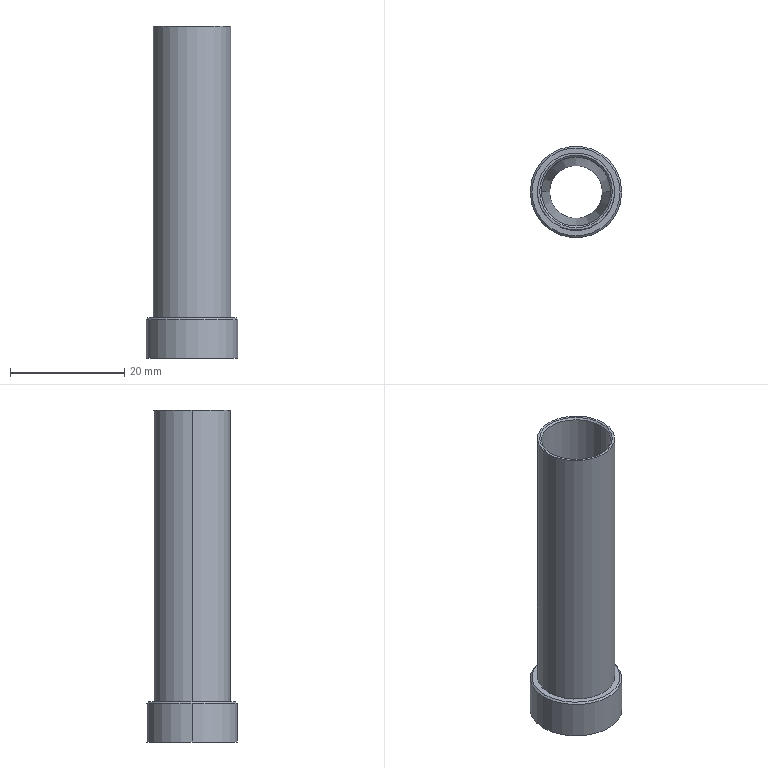Part | SolidWorks | features Chamfer 3, ICE 3, Extrusion 1 | 1 solid | 20 faces | box 16 x 16 x 58 mm | volume 2465 mm3 | cylinder 10 | cone 6 | plane 4 | commonest cylinder face diameters 9.2 x2 12.1 x2 12.5 x2 13.5 x2 16 x2
STEP:
#1=CARTESIAN_POINT('',(-6.05,0.,57.7));
#2=VERTEX_POINT('',#1);
#3=CARTESIAN_POINT('',(6.05,0.,57.7));
#4=VERTEX_POINT('',#3);
#5=CARTESIAN_POINT('',(0.,0.,57.7));
#6=DIRECTION('',(0.,0.,1.));
#7=DIRECTION('',(1.,0.,0.));
#8=AXIS2_PLACEMENT_3D('',#5,#6,#7);
#9=CIRCLE('',#8,6.05);
#10=EDGE_CURVE('',#2,#4,#9,.T.);
#11=ORIENTED_EDGE('',*,*,#10,.F.);
#12=CARTESIAN_POINT('',(-6.35,0.,58.));
#13=VERTEX_POINT('',#12);
#14=CARTESIAN_POINT('',(-6.05,0.,57.7));
#15=DIRECTION('',(-0.7071,0.,0.7071));
#16=VECTOR('',#15,1000.);
#17=LINE('',#14,#16);
#18=EDGE_CURVE('',#2,#13,#17,.T.);
#19=ORIENTED_EDGE('',*,*,#18,.T.);
#20=CARTESIAN_POINT('',(6.35,0.,58.));
#21=VERTEX_POINT('',#20);
#22=CARTESIAN_POINT('',(0.,0.,58.));
#23=DIRECTION('',(0.,0.,-1.));
#24=DIRECTION('',(1.,0.,0.));
#25=AXIS2_PLACEMENT_3D('',#22,#23,#24);
#26=CIRCLE('',#25,6.35);
#27=EDGE_CURVE('',#21,#13,#26,.T.);
#28=ORIENTED_EDGE('',*,*,#27,.F.);
#29=CARTESIAN_POINT('',(6.05,0.,57.7));
#30=DIRECTION('',(0.7071,0.,0.7071));
#31=VECTOR('',#30,1000.);
#32=LINE('',#29,#31);
#33=EDGE_CURVE('',#4,#21,#32,.T.);
#34=ORIENTED_EDGE('',*,*,#33,.F.);
#35=EDGE_LOOP('',(#11,#19,#28,#34));
#36=FACE_OUTER_BOUND('',#35,.T.);
#37=CARTESIAN_POINT('',(0.,0.,57.7));
#38=DIRECTION('',(0.,0.,1.));
#39=DIRECTION('',(1.,0.,0.));
#40=AXIS2_PLACEMENT_3D('',#37,#38,#39);
#41=CONICAL_SURFACE('',#40,6.05,0.7854);
#42=ADVANCED_FACE('',(#36),#41,.F.);
#43=CARTESIAN_POINT('',(-4.6,0.,8.));
#44=VERTEX_POINT('',#43);
#45=CARTESIAN_POINT('',(4.6,0.,8.));
#46=VERTEX_POINT('',#45);
#47=CARTESIAN_POINT('',(0.,0.,8.));
#48=DIRECTION('',(0.,0.,1.));
#49=DIRECTION('',(1.,0.,0.));
#50=AXIS2_PLACEMENT_3D('',#47,#48,#49);
#51=CIRCLE('',#50,4.6);
#52=EDGE_CURVE('',#44,#46,#51,.T.);
#53=ORIENTED_EDGE('',*,*,#52,.F.);
#54=CARTESIAN_POINT('',(-6.05,0.,23.));
#55=VERTEX_POINT('',#54);
#56=CARTESIAN_POINT('',(-4.6,0.,8.));
#57=DIRECTION('',(-0.09622,0.,0.9954));
#58=VECTOR('',#57,1000.);
#59=LINE('',#56,#58);
#60=EDGE_CURVE('',#44,#55,#59,.T.);
#61=ORIENTED_EDGE('',*,*,#60,.T.);
#62=CARTESIAN_POINT('',(6.05,0.,23.));
#63=VERTEX_POINT('',#62);
#64=CARTESIAN_POINT('',(0.,0.,23.));
#65=DIRECTION('',(0.,0.,1.));
#66=DIRECTION('',(1.,0.,0.));
#67=AXIS2_PLACEMENT_3D('',#64,#65,#66);
#68=CIRCLE('',#67,6.05);
#69=EDGE_CURVE('',#55,#63,#68,.T.);
#70=ORIENTED_EDGE('',*,*,#69,.T.);
#71=CARTESIAN_POINT('',(4.6,0.,8.));
#72=DIRECTION('',(0.09622,0.,0.9954));
#73=VECTOR('',#72,1000.);
#74=LINE('',#71,#73);
#75=EDGE_CURVE('',#46,#63,#74,.T.);
#76=ORIENTED_EDGE('',*,*,#75,.F.);
#77=EDGE_LOOP('',(#53,#61,#70,#76));
#78=FACE_OUTER_BOUND('',#77,.T.);
#79=CARTESIAN_POINT('',(0.,0.,8.));
#80=DIRECTION('',(0.,0.,1.));
#81=DIRECTION('',(1.,0.,0.));
#82=AXIS2_PLACEMENT_3D('',#79,#80,#81);
#83=CONICAL_SURFACE('',#82,4.6,0.09637);
#84=ADVANCED_FACE('',(#78),#83,.F.);
#85=ORIENTED_EDGE('',*,*,#69,.F.);
#86=CARTESIAN_POINT('',(-6.05,0.,23.));
#87=DIRECTION('',(0.,0.,1.));
#88=VECTOR('',#87,1000.);
#89=LINE('',#86,#88);
#90=EDGE_CURVE('',#55,#2,#89,.T.);
#91=ORIENTED_EDGE('',*,*,#90,.T.);
#92=ORIENTED_EDGE('',*,*,#10,.T.);
#93=CARTESIAN_POINT('',(6.05,0.,23.));
#94=DIRECTION('',(0.,0.,1.));
#95=VECTOR('',#94,1000.);
#96=LINE('',#93,#95);
#97=EDGE_CURVE('',#63,#4,#96,.T.);
#98=ORIENTED_EDGE('',*,*,#97,.F.);
#99=EDGE_LOOP('',(#85,#91,#92,#98));
#100=FACE_OUTER_BOUND('',#99,.T.);
#101=CARTESIAN_POINT('',(0.,0.,23.));
#102=DIRECTION('',(0.,0.,1.));
#103=DIRECTION('',(1.,0.,0.));
#104=AXIS2_PLACEMENT_3D('',#101,#102,#103);
#105=CYLINDRICAL_SURFACE('',#104,6.05);
#106=ADVANCED_FACE('',(#100),#105,.F.);
#107=CARTESIAN_POINT('',(7.7,0.,7.));
#108=VERTEX_POINT('',#107);
#109=CARTESIAN_POINT('',(-7.7,0.,7.));
#110=VERTEX_POINT('',#109);
#111=CARTESIAN_POINT('',(0.,0.,7.));
#112=DIRECTION('',(0.,0.,1.));
#113=DIRECTION('',(-1.,0.,0.));
#114=AXIS2_PLACEMENT_3D('',#111,#112,#113);
#115=CIRCLE('',#114,7.7);
#116=EDGE_CURVE('',#108,#110,#115,.T.);
#117=ORIENTED_EDGE('',*,*,#116,.F.);
#118=CARTESIAN_POINT('',(8.,0.,6.7));
#119=VERTEX_POINT('',#118);
#120=CARTESIAN_POINT('',(8.,0.,6.7));
#121=DIRECTION('',(0.7071,0.,-0.7071));
#122=VECTOR('',#121,1000.);
#123=LINE('',#120,#122);
#124=EDGE_CURVE('',#108,#119,#123,.T.);
#125=ORIENTED_EDGE('',*,*,#124,.T.);
#126=CARTESIAN_POINT('',(-8.,0.,6.7));
#127=VERTEX_POINT('',#126);
#128=CARTESIAN_POINT('',(0.,0.,6.7));
#129=DIRECTION('',(0.,0.,-1.));
#130=DIRECTION('',(-1.,0.,0.));
#131=AXIS2_PLACEMENT_3D('',#128,#129,#130);
#132=CIRCLE('',#131,8.);
#133=EDGE_CURVE('',#127,#119,#132,.T.);
#134=ORIENTED_EDGE('',*,*,#133,.F.);
#135=CARTESIAN_POINT('',(-8.,0.,6.7));
#136=DIRECTION('',(-0.7071,0.,-0.7071));
#137=VECTOR('',#136,1000.);
#138=LINE('',#135,#137);
#139=EDGE_CURVE('',#110,#127,#138,.T.);
#140=ORIENTED_EDGE('',*,*,#139,.F.);
#141=EDGE_LOOP('',(#117,#125,#134,#140));
#142=FACE_OUTER_BOUND('',#141,.T.);
#143=CARTESIAN_POINT('',(0.,0.,6.7));
#144=DIRECTION('',(0.,0.,-1.));
#145=DIRECTION('',(-1.,0.,0.));
#146=AXIS2_PLACEMENT_3D('',#143,#144,#145);
#147=CONICAL_SURFACE('',#146,8.,0.7854);
#148=ADVANCED_FACE('',(#142),#147,.T.);
#149=ORIENTED_EDGE('',*,*,#133,.T.);
#150=CARTESIAN_POINT('',(8.,0.,0.));
#151=VERTEX_POINT('',#150);
#152=CARTESIAN_POINT('',(8.,0.,7.));
#153=DIRECTION('',(0.,0.,-1.));
#154=VECTOR('',#153,1000.);
#155=LINE('',#152,#154);
#156=EDGE_CURVE('',#119,#151,#155,.T.);
#157=ORIENTED_EDGE('',*,*,#156,.T.);
#158=CARTESIAN_POINT('',(-8.,0.,0.));
#159=VERTEX_POINT('',#158);
#160=CARTESIAN_POINT('',(0.,0.,0.));
#161=DIRECTION('',(0.,0.,-1.));
#162=DIRECTION('',(-1.,0.,0.));
#163=AXIS2_PLACEMENT_3D('',#160,#161,#162);
#164=CIRCLE('',#163,8.);
#165=EDGE_CURVE('',#159,#151,#164,.T.);
#166=ORIENTED_EDGE('',*,*,#165,.F.);
#167=CARTESIAN_POINT('',(-8.,0.,7.));
#168=DIRECTION('',(0.,0.,-1.));
#169=VECTOR('',#168,1000.);
#170=LINE('',#167,#169);
#171=EDGE_CURVE('',#127,#159,#170,.T.);
#172=ORIENTED_EDGE('',*,*,#171,.F.);
#173=EDGE_LOOP('',(#149,#157,#166,#172));
#174=FACE_OUTER_BOUND('',#173,.T.);
#175=CARTESIAN_POINT('',(0.,0.,7.));
#176=DIRECTION('',(0.,0.,-1.));
#177=DIRECTION('',(-1.,0.,0.));
#178=AXIS2_PLACEMENT_3D('',#175,#176,#177);
#179=CYLINDRICAL_SURFACE('',#178,8.);
#180=ADVANCED_FACE('',(#174),#179,.T.);
#181=CARTESIAN_POINT('',(6.25,0.,6.));
#182=VERTEX_POINT('',#181);
#183=CARTESIAN_POINT('',(-6.25,0.,6.));
#184=VERTEX_POINT('',#183);
#185=CARTESIAN_POINT('',(0.,0.,6.));
#186=DIRECTION('',(0.,0.,-1.));
#187=DIRECTION('',(-1.,0.,0.));
#188=AXIS2_PLACEMENT_3D('',#185,#186,#187);
#189=CIRCLE('',#188,6.25);
#190=EDGE_CURVE('',#182,#184,#189,.T.);
#191=ORIENTED_EDGE('',*,*,#190,.F.);
#192=CARTESIAN_POINT('',(6.25,0.,0.));
#193=VERTEX_POINT('',#192);
#194=CARTESIAN_POINT('',(6.25,0.,6.));
#195=DIRECTION('',(0.,0.,-1.));
#196=VECTOR('',#195,1000.);
#197=LINE('',#194,#196);
#198=EDGE_CURVE('',#182,#193,#197,.T.);
#199=ORIENTED_EDGE('',*,*,#198,.T.);
#200=CARTESIAN_POINT('',(-6.25,0.,0.));
#201=VERTEX_POINT('',#200);
#202=CARTESIAN_POINT('',(0.,0.,0.));
#203=DIRECTION('',(0.,0.,-1.));
#204=DIRECTION('',(-1.,0.,0.));
#205=AXIS2_PLACEMENT_3D('',#202,#203,#204);
#206=CIRCLE('',#205,6.25);
#207=EDGE_CURVE('',#193,#201,#206,.T.);
#208=ORIENTED_EDGE('',*,*,#207,.T.);
#209=CARTESIAN_POINT('',(-6.25,0.,6.));
#210=DIRECTION('',(0.,0.,-1.));
#211=VECTOR('',#210,1000.);
#212=LINE('',#209,#211);
#213=EDGE_CURVE('',#184,#201,#212,.T.);
#214=ORIENTED_EDGE('',*,*,#213,.F.);
#215=EDGE_LOOP('',(#191,#199,#208,#214));
#216=FACE_OUTER_BOUND('',#215,.T.);
#217=CARTESIAN_POINT('',(0.,0.,6.));
#218=DIRECTION('',(0.,0.,-1.));
#219=DIRECTION('',(-1.,0.,0.));
#220=AXIS2_PLACEMENT_3D('',#217,#218,#219);
#221=CYLINDRICAL_SURFACE('',#220,6.25);
#222=ADVANCED_FACE('',(#216),#221,.F.);
#223=CARTESIAN_POINT('',(6.75,0.,58.));
#224=VERTEX_POINT('',#223);
#225=CARTESIAN_POINT('',(-6.75,0.,58.));
#226=VERTEX_POINT('',#225);
#227=CARTESIAN_POINT('',(0.,0.,58.));
#228=DIRECTION('',(0.,0.,1.));
#229=DIRECTION('',(1.,0.,0.));
#230=AXIS2_PLACEMENT_3D('',#227,#228,#229);
#231=CIRCLE('',#230,6.75);
#232=EDGE_CURVE('',#224,#226,#231,.T.);
#233=ORIENTED_EDGE('',*,*,#232,.F.);
#234=CARTESIAN_POINT('',(6.75,0.,7.));
#235=VERTEX_POINT('',#234);
#236=CARTESIAN_POINT('',(6.75,0.,58.));
#237=DIRECTION('',(0.,0.,-1.));
#238=VECTOR('',#237,1000.);
#239=LINE('',#236,#238);
#240=EDGE_CURVE('',#224,#235,#239,.T.);
#241=ORIENTED_EDGE('',*,*,#240,.T.);
#242=CARTESIAN_POINT('',(-6.75,0.,7.));
#243=VERTEX_POINT('',#242);
#244=CARTESIAN_POINT('',(0.,0.,7.));
#245=DIRECTION('',(0.,0.,-1.));
#246=DIRECTION('',(-1.,0.,0.));
#247=AXIS2_PLACEMENT_3D('',#244,#245,#246);
#248=CIRCLE('',#247,6.75);
#249=EDGE_CURVE('',#243,#235,#248,.T.);
#250=ORIENTED_EDGE('',*,*,#249,.F.);
#251=CARTESIAN_POINT('',(-6.75,0.,58.));
#252=DIRECTION('',(0.,0.,-1.));
#253=VECTOR('',#252,1000.);
#254=LINE('',#251,#253);
#255=EDGE_CURVE('',#226,#243,#254,.T.);
#256=ORIENTED_EDGE('',*,*,#255,.F.);
#257=EDGE_LOOP('',(#233,#241,#250,#256));
#258=FACE_OUTER_BOUND('',#257,.T.);
#259=CARTESIAN_POINT('',(0.,0.,58.));
#260=DIRECTION('',(0.,0.,-1.));
#261=DIRECTION('',(-1.,0.,0.));
#262=AXIS2_PLACEMENT_3D('',#259,#260,#261);
#263=CYLINDRICAL_SURFACE('',#262,6.75);
#264=ADVANCED_FACE('',(#258),#263,.T.);
#265=ORIENTED_EDGE('',*,*,#52,.T.);
#266=CARTESIAN_POINT('',(4.6,0.,6.));
#267=VERTEX_POINT('',#266);
#268=CARTESIAN_POINT('',(4.6,0.,58.));
#269=DIRECTION('',(0.,0.,-1.));
#270=VECTOR('',#269,1000.);
#271=LINE('',#268,#270);
#272=EDGE_CURVE('',#46,#267,#271,.T.);
#273=ORIENTED_EDGE('',*,*,#272,.T.);
#274=CARTESIAN_POINT('',(-4.6,0.,6.));
#275=VERTEX_POINT('',#274);
#276=CARTESIAN_POINT('',(0.,0.,6.));
#277=DIRECTION('',(0.,0.,-1.));
#278=DIRECTION('',(-1.,0.,0.));
#279=AXIS2_PLACEMENT_3D('',#276,#277,#278);
#280=CIRCLE('',#279,4.6);
#281=EDGE_CURVE('',#267,#275,#280,.T.);
#282=ORIENTED_EDGE('',*,*,#281,.T.);
#283=CARTESIAN_POINT('',(-4.6,0.,58.));
#284=DIRECTION('',(0.,0.,-1.));
#285=VECTOR('',#284,1000.);
#286=LINE('',#283,#285);
#287=EDGE_CURVE('',#44,#275,#286,.T.);
#288=ORIENTED_EDGE('',*,*,#287,.F.);
#289=EDGE_LOOP('',(#265,#273,#282,#288));
#290=FACE_OUTER_BOUND('',#289,.T.);
#291=CARTESIAN_POINT('',(0.,0.,58.));
#292=DIRECTION('',(0.,0.,-1.));
#293=DIRECTION('',(-1.,0.,0.));
#294=AXIS2_PLACEMENT_3D('',#291,#292,#293);
#295=CYLINDRICAL_SURFACE('',#294,4.6);
#296=ADVANCED_FACE('',(#290),#295,.F.);
#297=ORIENTED_EDGE('',*,*,#272,.F.);
#298=CARTESIAN_POINT('',(0.,0.,8.));
#299=DIRECTION('',(0.,0.,1.));
#300=DIRECTION('',(1.,0.,0.));
#301=AXIS2_PLACEMENT_3D('',#298,#299,#300);
#302=CIRCLE('',#301,4.6);
#303=EDGE_CURVE('',#46,#44,#302,.T.);
#304=ORIENTED_EDGE('',*,*,#303,.T.);
#305=ORIENTED_EDGE('',*,*,#287,.T.);
#306=CARTESIAN_POINT('',(0.,0.,6.));
#307=DIRECTION('',(0.,0.,-1.));
#308=DIRECTION('',(-1.,0.,0.));
#309=AXIS2_PLACEMENT_3D('',#306,#307,#308);
#310=CIRCLE('',#309,4.6);
#311=EDGE_CURVE('',#275,#267,#310,.T.);
#312=ORIENTED_EDGE('',*,*,#311,.T.);
#313=EDGE_LOOP('',(#297,#304,#305,#312));
#314=FACE_OUTER_BOUND('',#313,.T.);
#315=CARTESIAN_POINT('',(0.,0.,58.));
#316=DIRECTION('',(0.,0.,-1.));
#317=DIRECTION('',(-1.,0.,0.));
#318=AXIS2_PLACEMENT_3D('',#315,#316,#317);
#319=CYLINDRICAL_SURFACE('',#318,4.6);
#320=ADVANCED_FACE('',(#314),#319,.F.);
#321=ORIENTED_EDGE('',*,*,#240,.F.);
#322=CARTESIAN_POINT('',(0.,0.,58.));
#323=DIRECTION('',(0.,0.,1.));
#324=DIRECTION('',(1.,0.,0.));
#325=AXIS2_PLACEMENT_3D('',#322,#323,#324);
#326=CIRCLE('',#325,6.75);
#327=EDGE_CURVE('',#226,#224,#326,.T.);
#328=ORIENTED_EDGE('',*,*,#327,.F.);
#329=ORIENTED_EDGE('',*,*,#255,.T.);
#330=CARTESIAN_POINT('',(0.,0.,7.));
#331=DIRECTION('',(0.,0.,-1.));
#332=DIRECTION('',(-1.,0.,0.));
#333=AXIS2_PLACEMENT_3D('',#330,#331,#332);
#334=CIRCLE('',#333,6.75);
#335=EDGE_CURVE('',#235,#243,#334,.T.);
#336=ORIENTED_EDGE('',*,*,#335,.F.);
#337=EDGE_LOOP('',(#321,#328,#329,#336));
#338=FACE_OUTER_BOUND('',#337,.T.);
#339=CARTESIAN_POINT('',(0.,0.,58.));
#340=DIRECTION('',(0.,0.,-1.));
#341=DIRECTION('',(-1.,0.,0.));
#342=AXIS2_PLACEMENT_3D('',#339,#340,#341);
#343=CYLINDRICAL_SURFACE('',#342,6.75);
#344=ADVANCED_FACE('',(#338),#343,.T.);
#345=ORIENTED_EDGE('',*,*,#27,.T.);
#346=CARTESIAN_POINT('',(0.,0.,58.));
#347=DIRECTION('',(0.,0.,-1.));
#348=DIRECTION('',(1.,0.,0.));
#349=AXIS2_PLACEMENT_3D('',#346,#347,#348);
#350=CIRCLE('',#349,6.35);
#351=EDGE_CURVE('',#13,#21,#350,.T.);
#352=ORIENTED_EDGE('',*,*,#351,.T.);
#353=EDGE_LOOP('',(#345,#352));
#354=FACE_BOUND('',#353,.T.);
#355=ORIENTED_EDGE('',*,*,#327,.T.);
#356=ORIENTED_EDGE('',*,*,#232,.T.);
#357=EDGE_LOOP('',(#355,#356));
#358=FACE_OUTER_BOUND('',#357,.T.);
#359=CARTESIAN_POINT('',(0.,0.,58.));
#360=DIRECTION('',(0.,0.,1.));
#361=DIRECTION('',(1.,0.,0.));
#362=AXIS2_PLACEMENT_3D('',#359,#360,#361);
#363=PLANE('',#362);
#364=ADVANCED_FACE('',(#354,#358),#363,.T.);
#365=CARTESIAN_POINT('',(0.,0.,0.));
#366=DIRECTION('',(0.,0.,-1.));
#367=DIRECTION('',(-1.,0.,0.));
#368=AXIS2_PLACEMENT_3D('',#365,#366,#367);
#369=CIRCLE('',#368,6.25);
#370=EDGE_CURVE('',#201,#193,#369,.T.);
#371=ORIENTED_EDGE('',*,*,#370,.F.);
#372=ORIENTED_EDGE('',*,*,#207,.F.);
#373=EDGE_LOOP('',(#371,#372));
#374=FACE_BOUND('',#373,.T.);
#375=ORIENTED_EDGE('',*,*,#165,.T.);
#376=CARTESIAN_POINT('',(0.,0.,0.));
#377=DIRECTION('',(0.,0.,-1.));
#378=DIRECTION('',(-1.,0.,0.));
#379=AXIS2_PLACEMENT_3D('',#376,#377,#378);
#380=CIRCLE('',#379,8.);
#381=EDGE_CURVE('',#151,#159,#380,.T.);
#382=ORIENTED_EDGE('',*,*,#381,.T.);
#383=EDGE_LOOP('',(#375,#382));
#384=FACE_OUTER_BOUND('',#383,.T.);
#385=CARTESIAN_POINT('',(0.,0.,0.));
#386=DIRECTION('',(0.,0.,1.));
#387=DIRECTION('',(1.,0.,0.));
#388=AXIS2_PLACEMENT_3D('',#385,#386,#387);
#389=PLANE('',#388);
#390=ADVANCED_FACE('',(#374,#384),#389,.F.);
#391=ORIENTED_EDGE('',*,*,#198,.F.);
#392=CARTESIAN_POINT('',(0.,0.,6.));
#393=DIRECTION('',(0.,0.,-1.));
#394=DIRECTION('',(-1.,0.,0.));
#395=AXIS2_PLACEMENT_3D('',#392,#393,#394);
#396=CIRCLE('',#395,6.25);
#397=EDGE_CURVE('',#184,#182,#396,.T.);
#398=ORIENTED_EDGE('',*,*,#397,.F.);
#399=ORIENTED_EDGE('',*,*,#213,.T.);
#400=ORIENTED_EDGE('',*,*,#370,.T.);
#401=EDGE_LOOP('',(#391,#398,#399,#400));
#402=FACE_OUTER_BOUND('',#401,.T.);
#403=CARTESIAN_POINT('',(0.,0.,6.));
#404=DIRECTION('',(0.,0.,-1.));
#405=DIRECTION('',(-1.,0.,0.));
#406=AXIS2_PLACEMENT_3D('',#403,#404,#405);
#407=CYLINDRICAL_SURFACE('',#406,6.25);
#408=ADVANCED_FACE('',(#402),#407,.F.);
#409=ORIENTED_EDGE('',*,*,#311,.F.);
#410=ORIENTED_EDGE('',*,*,#281,.F.);
#411=EDGE_LOOP('',(#409,#410));
#412=FACE_BOUND('',#411,.T.);
#413=ORIENTED_EDGE('',*,*,#397,.T.);
#414=ORIENTED_EDGE('',*,*,#190,.T.);
#415=EDGE_LOOP('',(#413,#414));
#416=FACE_OUTER_BOUND('',#415,.T.);
#417=CARTESIAN_POINT('',(0.,0.,6.));
#418=DIRECTION('',(0.,0.,-1.));
#419=DIRECTION('',(-1.,0.,0.));
#420=AXIS2_PLACEMENT_3D('',#417,#418,#419);
#421=PLANE('',#420);
#422=ADVANCED_FACE('',(#412,#416),#421,.T.);
#423=ORIENTED_EDGE('',*,*,#156,.F.);
#424=CARTESIAN_POINT('',(0.,0.,6.7));
#425=DIRECTION('',(0.,0.,-1.));
#426=DIRECTION('',(-1.,0.,0.));
#427=AXIS2_PLACEMENT_3D('',#424,#425,#426);
#428=CIRCLE('',#427,8.);
#429=EDGE_CURVE('',#119,#127,#428,.T.);
#430=ORIENTED_EDGE('',*,*,#429,.T.);
#431=ORIENTED_EDGE('',*,*,#171,.T.);
#432=ORIENTED_EDGE('',*,*,#381,.F.);
#433=EDGE_LOOP('',(#423,#430,#431,#432));
#434=FACE_OUTER_BOUND('',#433,.T.);
#435=CARTESIAN_POINT('',(0.,0.,7.));
#436=DIRECTION('',(0.,0.,-1.));
#437=DIRECTION('',(-1.,0.,0.));
#438=AXIS2_PLACEMENT_3D('',#435,#436,#437);
#439=CYLINDRICAL_SURFACE('',#438,8.);
#440=ADVANCED_FACE('',(#434),#439,.T.);
#441=CARTESIAN_POINT('',(0.,0.,7.));
#442=DIRECTION('',(0.,0.,1.));
#443=DIRECTION('',(-1.,0.,0.));
#444=AXIS2_PLACEMENT_3D('',#441,#442,#443);
#445=CIRCLE('',#444,7.7);
#446=EDGE_CURVE('',#110,#108,#445,.T.);
#447=ORIENTED_EDGE('',*,*,#446,.T.);
#448=ORIENTED_EDGE('',*,*,#116,.T.);
#449=EDGE_LOOP('',(#447,#448));
#450=FACE_OUTER_BOUND('',#449,.T.);
#451=ORIENTED_EDGE('',*,*,#249,.T.);
#452=ORIENTED_EDGE('',*,*,#335,.T.);
#453=EDGE_LOOP('',(#451,#452));
#454=FACE_BOUND('',#453,.T.);
#455=CARTESIAN_POINT('',(0.,0.,7.));
#456=DIRECTION('',(0.,0.,-1.));
#457=DIRECTION('',(-1.,0.,0.));
#458=AXIS2_PLACEMENT_3D('',#455,#456,#457);
#459=PLANE('',#458);
#460=ADVANCED_FACE('',(#450,#454),#459,.F.);
#461=ORIENTED_EDGE('',*,*,#124,.F.);
#462=ORIENTED_EDGE('',*,*,#446,.F.);
#463=ORIENTED_EDGE('',*,*,#139,.T.);
#464=ORIENTED_EDGE('',*,*,#429,.F.);
#465=EDGE_LOOP('',(#461,#462,#463,#464));
#466=FACE_OUTER_BOUND('',#465,.T.);
#467=CARTESIAN_POINT('',(0.,0.,6.7));
#468=DIRECTION('',(0.,0.,-1.));
#469=DIRECTION('',(-1.,0.,0.));
#470=AXIS2_PLACEMENT_3D('',#467,#468,#469);
#471=CONICAL_SURFACE('',#470,8.,0.7854);
#472=ADVANCED_FACE('',(#466),#471,.T.);
#473=ORIENTED_EDGE('',*,*,#90,.F.);
#474=CARTESIAN_POINT('',(0.,0.,23.));
#475=DIRECTION('',(0.,0.,1.));
#476=DIRECTION('',(1.,0.,0.));
#477=AXIS2_PLACEMENT_3D('',#474,#475,#476);
#478=CIRCLE('',#477,6.05);
#479=EDGE_CURVE('',#63,#55,#478,.T.);
#480=ORIENTED_EDGE('',*,*,#479,.F.);
#481=ORIENTED_EDGE('',*,*,#97,.T.);
#482=CARTESIAN_POINT('',(0.,0.,57.7));
#483=DIRECTION('',(0.,0.,1.));
#484=DIRECTION('',(1.,0.,0.));
#485=AXIS2_PLACEMENT_3D('',#482,#483,#484);
#486=CIRCLE('',#485,6.05);
#487=EDGE_CURVE('',#4,#2,#486,.T.);
#488=ORIENTED_EDGE('',*,*,#487,.T.);
#489=EDGE_LOOP('',(#473,#480,#481,#488));
#490=FACE_OUTER_BOUND('',#489,.T.);
#491=CARTESIAN_POINT('',(0.,0.,23.));
#492=DIRECTION('',(0.,0.,1.));
#493=DIRECTION('',(1.,0.,0.));
#494=AXIS2_PLACEMENT_3D('',#491,#492,#493);
#495=CYLINDRICAL_SURFACE('',#494,6.05);
#496=ADVANCED_FACE('',(#490),#495,.F.);
#497=ORIENTED_EDGE('',*,*,#60,.F.);
#498=ORIENTED_EDGE('',*,*,#303,.F.);
#499=ORIENTED_EDGE('',*,*,#75,.T.);
#500=ORIENTED_EDGE('',*,*,#479,.T.);
#501=EDGE_LOOP('',(#497,#498,#499,#500));
#502=FACE_OUTER_BOUND('',#501,.T.);
#503=CARTESIAN_POINT('',(0.,0.,8.));
#504=DIRECTION('',(0.,0.,1.));
#505=DIRECTION('',(1.,0.,0.));
#506=AXIS2_PLACEMENT_3D('',#503,#504,#505);
#507=CONICAL_SURFACE('',#506,4.6,0.09637);
#508=ADVANCED_FACE('',(#502),#507,.F.);
#509=ORIENTED_EDGE('',*,*,#18,.F.);
#510=ORIENTED_EDGE('',*,*,#487,.F.);
#511=ORIENTED_EDGE('',*,*,#33,.T.);
#512=ORIENTED_EDGE('',*,*,#351,.F.);
#513=EDGE_LOOP('',(#509,#510,#511,#512));
#514=FACE_OUTER_BOUND('',#513,.T.);
#515=CARTESIAN_POINT('',(0.,0.,57.7));
#516=DIRECTION('',(0.,0.,1.));
#517=DIRECTION('',(1.,0.,0.));
#518=AXIS2_PLACEMENT_3D('',#515,#516,#517);
#519=CONICAL_SURFACE('',#518,6.05,0.7854);
#520=ADVANCED_FACE('',(#514),#519,.F.);
#521=CLOSED_SHELL('',(#42,#84,#106,#148,#180,#222,#264,#296,#320,#344,#364,#390,#408,#422,#440,#460,#472,#496,#508,#520));
#522=MANIFOLD_SOLID_BREP('',#521);
#523=CARTESIAN_POINT('',(0.,0.,0.));
#524=DIRECTION('',(0.,0.,1.));
#525=DIRECTION('',(1.,0.,0.));
#526=AXIS2_PLACEMENT_3D('',#523,#524,#525);
#527=(LENGTH_UNIT()NAMED_UNIT(*)SI_UNIT(.MILLI.,.METRE.));
#528=UNCERTAINTY_MEASURE_WITH_UNIT(LENGTH_MEASURE(0.00001),#527,'','');
#529=(NAMED_UNIT(*)PLANE_ANGLE_UNIT()SI_UNIT($,.RADIAN.));
#530=(NAMED_UNIT(*)SI_UNIT($,.STERADIAN.)SOLID_ANGLE_UNIT());
#531=(GEOMETRIC_REPRESENTATION_CONTEXT(3)GLOBAL_UNCERTAINTY_ASSIGNED_CONTEXT((#528))GLOBAL_UNIT_ASSIGNED_CONTEXT((#527,#529,#530))REPRESENTATION_CONTEXT('',''));
#532=ADVANCED_BREP_SHAPE_REPRESENTATION('',(#522,#526),#531);